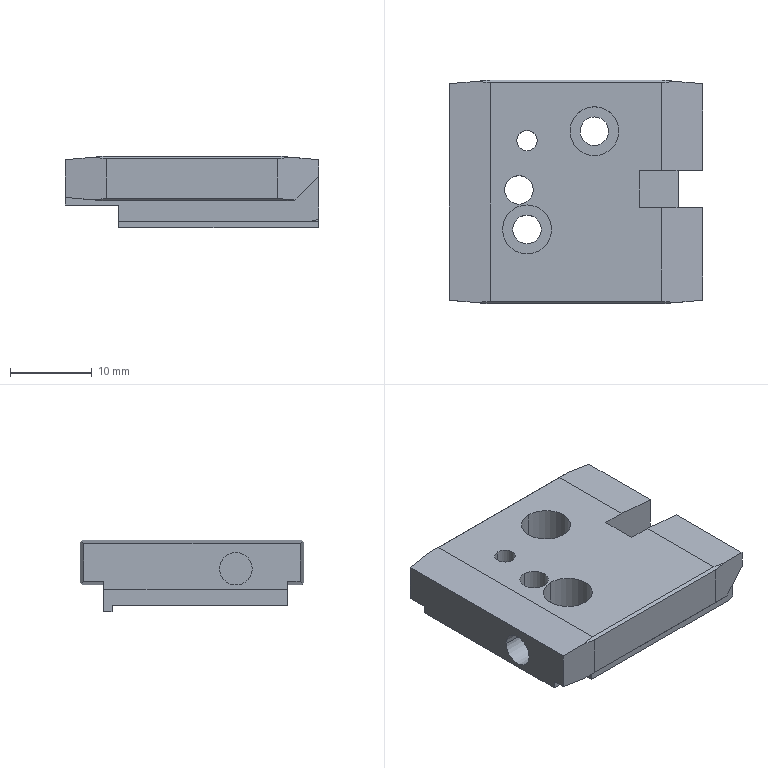Part | NX | 1 solid | 64 faces | box 31 x 27.4 x 8.8 mm | volume 5388 mm3 | plane 46 | cylinder 18 | commonest cylinder face diameters 3.5 x6 0.8 x4 6 x4 2.5 x2 4 x2